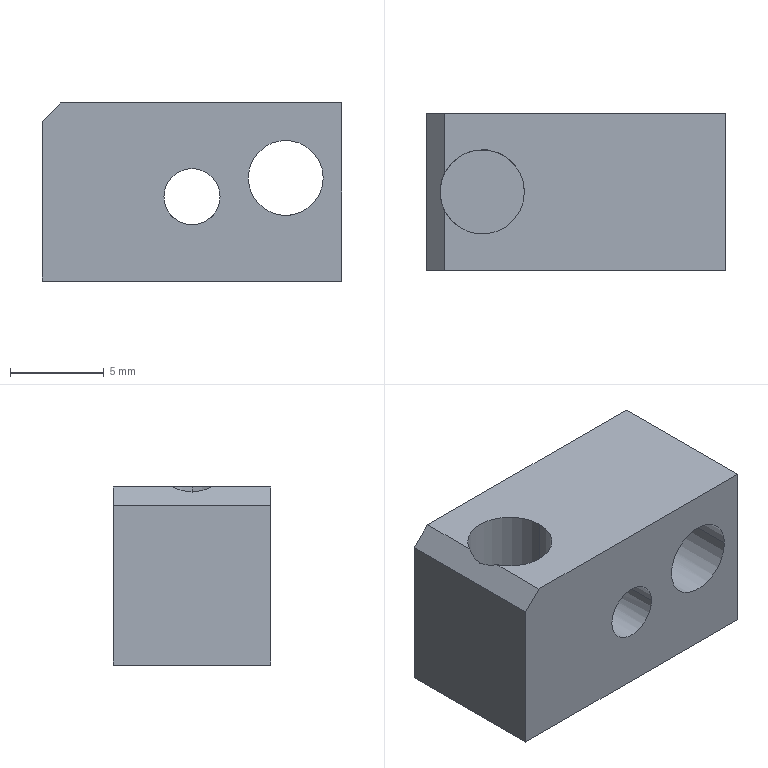Part | NX | 1 solid | 22 faces | box 16 x 8.4 x 9.5 mm | volume 978.124 mm3 | cylinder 10 | plane 8 | cone 4 | commonest cylinder face diameters 2.5 x4 3 x2 4 x2 4.5 x2
STEP:
#1=CARTESIAN_POINT('',(-8.,-4.2,-4.75));
#2=VERTEX_POINT('',#1);
#3=CARTESIAN_POINT('',(-8.,4.2,-4.75));
#4=VERTEX_POINT('',#3);
#5=CARTESIAN_POINT('',(-8.,0.,-4.75));
#6=DIRECTION('',(0.,1.,0.));
#7=VECTOR('',#6,1000.);
#8=LINE('',#5,#7);
#9=EDGE_CURVE('',#2,#4,#8,.T.);
#10=ORIENTED_EDGE('',*,*,#9,.T.);
#11=CARTESIAN_POINT('',(8.,4.2,-4.75));
#12=VERTEX_POINT('',#11);
#13=CARTESIAN_POINT('',(0.,4.2,-4.75));
#14=DIRECTION('',(1.,0.,0.));
#15=VECTOR('',#14,1000.);
#16=LINE('',#13,#15);
#17=EDGE_CURVE('',#4,#12,#16,.T.);
#18=ORIENTED_EDGE('',*,*,#17,.T.);
#19=CARTESIAN_POINT('',(8.,-4.2,-4.75));
#20=VERTEX_POINT('',#19);
#21=CARTESIAN_POINT('',(8.,0.,-4.75));
#22=DIRECTION('',(0.,-1.,0.));
#23=VECTOR('',#22,1000.);
#24=LINE('',#21,#23);
#25=EDGE_CURVE('',#12,#20,#24,.T.);
#26=ORIENTED_EDGE('',*,*,#25,.T.);
#27=CARTESIAN_POINT('',(0.,-4.2,-4.75));
#28=DIRECTION('',(-1.,0.,0.));
#29=VECTOR('',#28,1000.);
#30=LINE('',#27,#29);
#31=EDGE_CURVE('',#20,#2,#30,.T.);
#32=ORIENTED_EDGE('',*,*,#31,.T.);
#33=EDGE_LOOP('',(#10,#18,#26,#32));
#34=FACE_BOUND('',#33,.T.);
#35=CARTESIAN_POINT('',(3.3,0.,-4.75));
#36=VERTEX_POINT('',#35);
#37=CARTESIAN_POINT('',(6.7,0.,-4.75));
#38=VERTEX_POINT('',#37);
#39=CARTESIAN_POINT('',(5.,0.,-4.75));
#40=DIRECTION('',(0.,0.,-1.));
#41=DIRECTION('',(-1.,0.,0.));
#42=AXIS2_PLACEMENT_3D('',#39,#40,#41);
#43=CIRCLE('',#42,1.7);
#44=EDGE_CURVE('',#36,#38,#43,.T.);
#45=ORIENTED_EDGE('',*,*,#44,.F.);
#46=CARTESIAN_POINT('',(5.,0.,-4.75));
#47=DIRECTION('',(0.,0.,-1.));
#48=DIRECTION('',(-1.,0.,0.));
#49=AXIS2_PLACEMENT_3D('',#46,#47,#48);
#50=CIRCLE('',#49,1.7);
#51=EDGE_CURVE('',#38,#36,#50,.T.);
#52=ORIENTED_EDGE('',*,*,#51,.F.);
#53=EDGE_LOOP('',(#45,#52));
#54=FACE_BOUND('',#53,.T.);
#55=CARTESIAN_POINT('',(1.7,0.,-4.75));
#56=VERTEX_POINT('',#55);
#57=CARTESIAN_POINT('',(-1.7,0.,-4.75));
#58=VERTEX_POINT('',#57);
#59=CARTESIAN_POINT('',(0.,0.,-4.75));
#60=DIRECTION('',(0.,0.,-1.));
#61=DIRECTION('',(-1.,0.,0.));
#62=AXIS2_PLACEMENT_3D('',#59,#60,#61);
#63=CIRCLE('',#62,1.7);
#64=EDGE_CURVE('',#56,#58,#63,.T.);
#65=ORIENTED_EDGE('',*,*,#64,.F.);
#66=CARTESIAN_POINT('',(0.,0.,-4.75));
#67=DIRECTION('',(0.,0.,-1.));
#68=DIRECTION('',(-1.,0.,0.));
#69=AXIS2_PLACEMENT_3D('',#66,#67,#68);
#70=CIRCLE('',#69,1.7);
#71=EDGE_CURVE('',#58,#56,#70,.T.);
#72=ORIENTED_EDGE('',*,*,#71,.F.);
#73=EDGE_LOOP('',(#65,#72));
#74=FACE_BOUND('',#73,.T.);
#75=CARTESIAN_POINT('',(0.,0.,-4.75));
#76=DIRECTION('',(0.,0.,1.));
#77=DIRECTION('',(1.,0.,0.));
#78=AXIS2_PLACEMENT_3D('',#75,#76,#77);
#79=PLANE('',#78);
#80=ADVANCED_FACE('',(#34,#54,#74),#79,.F.);
#81=ORIENTED_EDGE('',*,*,#9,.F.);
#82=CARTESIAN_POINT('',(-8.,-4.2,3.75));
#83=VERTEX_POINT('',#82);
#84=CARTESIAN_POINT('',(-8.,-4.2,3.75));
#85=DIRECTION('',(0.,0.,-1.));
#86=VECTOR('',#85,1000.);
#87=LINE('',#84,#86);
#88=EDGE_CURVE('',#83,#2,#87,.T.);
#89=ORIENTED_EDGE('',*,*,#88,.F.);
#90=CARTESIAN_POINT('',(-8.,4.2,3.75));
#91=VERTEX_POINT('',#90);
#92=CARTESIAN_POINT('',(-8.,-4.2,3.75));
#93=DIRECTION('',(0.,1.,0.));
#94=VECTOR('',#93,1000.);
#95=LINE('',#92,#94);
#96=EDGE_CURVE('',#83,#91,#95,.T.);
#97=ORIENTED_EDGE('',*,*,#96,.T.);
#98=CARTESIAN_POINT('',(-8.,4.2,3.75));
#99=DIRECTION('',(0.,0.,-1.));
#100=VECTOR('',#99,1000.);
#101=LINE('',#98,#100);
#102=EDGE_CURVE('',#91,#4,#101,.T.);
#103=ORIENTED_EDGE('',*,*,#102,.T.);
#104=EDGE_LOOP('',(#81,#89,#97,#103));
#105=FACE_BOUND('',#104,.T.);
#106=CARTESIAN_POINT('',(-8.,4.2,-4.75));
#107=DIRECTION('',(-1.,0.,0.));
#108=DIRECTION('',(0.,0.,1.));
#109=AXIS2_PLACEMENT_3D('',#106,#107,#108);
#110=PLANE('',#109);
#111=ADVANCED_FACE('',(#105),#110,.T.);
#112=ORIENTED_EDGE('',*,*,#17,.F.);
#113=ORIENTED_EDGE('',*,*,#102,.F.);
#114=CARTESIAN_POINT('',(-7.,4.2,4.75));
#115=VERTEX_POINT('',#114);
#116=CARTESIAN_POINT('',(-7.,4.2,4.75));
#117=DIRECTION('',(-0.7071,0.,-0.7071));
#118=VECTOR('',#117,1000.);
#119=LINE('',#116,#118);
#120=EDGE_CURVE('',#115,#91,#119,.T.);
#121=ORIENTED_EDGE('',*,*,#120,.F.);
#122=CARTESIAN_POINT('',(8.,4.2,4.75));
#123=VERTEX_POINT('',#122);
#124=CARTESIAN_POINT('',(-7.,4.2,4.75));
#125=DIRECTION('',(1.,0.,0.));
#126=VECTOR('',#125,1000.);
#127=LINE('',#124,#126);
#128=EDGE_CURVE('',#115,#123,#127,.T.);
#129=ORIENTED_EDGE('',*,*,#128,.T.);
#130=CARTESIAN_POINT('',(8.,4.2,4.75));
#131=DIRECTION('',(0.,0.,-1.));
#132=VECTOR('',#131,1000.);
#133=LINE('',#130,#132);
#134=EDGE_CURVE('',#123,#12,#133,.T.);
#135=ORIENTED_EDGE('',*,*,#134,.T.);
#136=EDGE_LOOP('',(#112,#113,#121,#129,#135));
#137=FACE_BOUND('',#136,.T.);
#138=CARTESIAN_POINT('',(7.,4.2,0.75));
#139=VERTEX_POINT('',#138);
#140=CARTESIAN_POINT('',(3.,4.2,0.75));
#141=VERTEX_POINT('',#140);
#142=CARTESIAN_POINT('',(5.,4.2,0.75));
#143=DIRECTION('',(0.,1.,0.));
#144=DIRECTION('',(-1.,0.,0.));
#145=AXIS2_PLACEMENT_3D('',#142,#143,#144);
#146=CIRCLE('',#145,2.);
#147=EDGE_CURVE('',#139,#141,#146,.T.);
#148=ORIENTED_EDGE('',*,*,#147,.F.);
#149=CARTESIAN_POINT('',(5.,4.2,0.75));
#150=DIRECTION('',(0.,1.,0.));
#151=DIRECTION('',(-1.,0.,0.));
#152=AXIS2_PLACEMENT_3D('',#149,#150,#151);
#153=CIRCLE('',#152,2.);
#154=EDGE_CURVE('',#141,#139,#153,.T.);
#155=ORIENTED_EDGE('',*,*,#154,.F.);
#156=EDGE_LOOP('',(#148,#155));
#157=FACE_BOUND('',#156,.T.);
#158=CARTESIAN_POINT('',(-1.5,4.2,-0.25));
#159=VERTEX_POINT('',#158);
#160=CARTESIAN_POINT('',(1.5,4.2,-0.25));
#161=VERTEX_POINT('',#160);
#162=CARTESIAN_POINT('',(0.,4.2,-0.25));
#163=DIRECTION('',(0.,1.,0.));
#164=DIRECTION('',(-1.,0.,0.));
#165=AXIS2_PLACEMENT_3D('',#162,#163,#164);
#166=CIRCLE('',#165,1.5);
#167=EDGE_CURVE('',#159,#161,#166,.T.);
#168=ORIENTED_EDGE('',*,*,#167,.F.);
#169=CARTESIAN_POINT('',(0.,4.2,-0.25));
#170=DIRECTION('',(0.,1.,0.));
#171=DIRECTION('',(-1.,0.,0.));
#172=AXIS2_PLACEMENT_3D('',#169,#170,#171);
#173=CIRCLE('',#172,1.5);
#174=EDGE_CURVE('',#161,#159,#173,.T.);
#175=ORIENTED_EDGE('',*,*,#174,.F.);
#176=EDGE_LOOP('',(#168,#175));
#177=FACE_BOUND('',#176,.T.);
#178=CARTESIAN_POINT('',(8.,4.2,-4.75));
#179=DIRECTION('',(0.,1.,0.));
#180=DIRECTION('',(1.,0.,0.));
#181=AXIS2_PLACEMENT_3D('',#178,#179,#180);
#182=PLANE('',#181);
#183=ADVANCED_FACE('',(#137,#157,#177),#182,.T.);
#184=ORIENTED_EDGE('',*,*,#25,.F.);
#185=ORIENTED_EDGE('',*,*,#134,.F.);
#186=CARTESIAN_POINT('',(8.,-4.2,4.75));
#187=VERTEX_POINT('',#186);
#188=CARTESIAN_POINT('',(8.,4.2,4.75));
#189=DIRECTION('',(0.,-1.,0.));
#190=VECTOR('',#189,1000.);
#191=LINE('',#188,#190);
#192=EDGE_CURVE('',#123,#187,#191,.T.);
#193=ORIENTED_EDGE('',*,*,#192,.T.);
#194=CARTESIAN_POINT('',(8.,-4.2,4.75));
#195=DIRECTION('',(0.,0.,-1.));
#196=VECTOR('',#195,1000.);
#197=LINE('',#194,#196);
#198=EDGE_CURVE('',#187,#20,#197,.T.);
#199=ORIENTED_EDGE('',*,*,#198,.T.);
#200=EDGE_LOOP('',(#184,#185,#193,#199));
#201=FACE_BOUND('',#200,.T.);
#202=CARTESIAN_POINT('',(8.,-4.2,-4.75));
#203=DIRECTION('',(1.,0.,0.));
#204=DIRECTION('',(0.,1.,0.));
#205=AXIS2_PLACEMENT_3D('',#202,#203,#204);
#206=PLANE('',#205);
#207=ADVANCED_FACE('',(#201),#206,.T.);
#208=ORIENTED_EDGE('',*,*,#31,.F.);
#209=ORIENTED_EDGE('',*,*,#198,.F.);
#210=CARTESIAN_POINT('',(-7.,-4.2,4.75));
#211=VERTEX_POINT('',#210);
#212=CARTESIAN_POINT('',(8.,-4.2,4.75));
#213=DIRECTION('',(-1.,0.,0.));
#214=VECTOR('',#213,1000.);
#215=LINE('',#212,#214);
#216=EDGE_CURVE('',#187,#211,#215,.T.);
#217=ORIENTED_EDGE('',*,*,#216,.T.);
#218=CARTESIAN_POINT('',(-8.,-4.2,3.75));
#219=DIRECTION('',(0.7071,0.,0.7071));
#220=VECTOR('',#219,1000.);
#221=LINE('',#218,#220);
#222=EDGE_CURVE('',#83,#211,#221,.T.);
#223=ORIENTED_EDGE('',*,*,#222,.F.);
#224=ORIENTED_EDGE('',*,*,#88,.T.);
#225=EDGE_LOOP('',(#208,#209,#217,#223,#224));
#226=FACE_BOUND('',#225,.T.);
#227=CARTESIAN_POINT('',(7.,-4.2,0.75));
#228=VERTEX_POINT('',#227);
#229=CARTESIAN_POINT('',(3.,-4.2,0.75));
#230=VERTEX_POINT('',#229);
#231=CARTESIAN_POINT('',(5.,-4.2,0.75));
#232=DIRECTION('',(0.,1.,0.));
#233=DIRECTION('',(-1.,0.,0.));
#234=AXIS2_PLACEMENT_3D('',#231,#232,#233);
#235=CIRCLE('',#234,2.);
#236=EDGE_CURVE('',#228,#230,#235,.T.);
#237=ORIENTED_EDGE('',*,*,#236,.T.);
#238=CARTESIAN_POINT('',(5.,-4.2,0.75));
#239=DIRECTION('',(0.,1.,0.));
#240=DIRECTION('',(-1.,0.,0.));
#241=AXIS2_PLACEMENT_3D('',#238,#239,#240);
#242=CIRCLE('',#241,2.);
#243=EDGE_CURVE('',#230,#228,#242,.T.);
#244=ORIENTED_EDGE('',*,*,#243,.T.);
#245=EDGE_LOOP('',(#237,#244));
#246=FACE_BOUND('',#245,.T.);
#247=CARTESIAN_POINT('',(-1.5,-4.2,-0.25));
#248=VERTEX_POINT('',#247);
#249=CARTESIAN_POINT('',(1.5,-4.2,-0.25));
#250=VERTEX_POINT('',#249);
#251=CARTESIAN_POINT('',(0.,-4.2,-0.25));
#252=DIRECTION('',(0.,1.,0.));
#253=DIRECTION('',(-1.,0.,0.));
#254=AXIS2_PLACEMENT_3D('',#251,#252,#253);
#255=CIRCLE('',#254,1.5);
#256=EDGE_CURVE('',#248,#250,#255,.T.);
#257=ORIENTED_EDGE('',*,*,#256,.T.);
#258=CARTESIAN_POINT('',(0.,-4.2,-0.25));
#259=DIRECTION('',(0.,1.,0.));
#260=DIRECTION('',(-1.,0.,0.));
#261=AXIS2_PLACEMENT_3D('',#258,#259,#260);
#262=CIRCLE('',#261,1.5);
#263=EDGE_CURVE('',#250,#248,#262,.T.);
#264=ORIENTED_EDGE('',*,*,#263,.T.);
#265=EDGE_LOOP('',(#257,#264));
#266=FACE_BOUND('',#265,.T.);
#267=CARTESIAN_POINT('',(-8.,-4.2,-4.75));
#268=DIRECTION('',(0.,-1.,0.));
#269=DIRECTION('',(0.,0.,-1.));
#270=AXIS2_PLACEMENT_3D('',#267,#268,#269);
#271=PLANE('',#270);
#272=ADVANCED_FACE('',(#226,#246,#266),#271,.T.);
#273=CARTESIAN_POINT('',(-7.25,0.,4.5));
#274=VERTEX_POINT('',#273);
#275=CARTESIAN_POINT('',(-7.,-1.031,4.75));
#276=VERTEX_POINT('',#275);
#277=CARTESIAN_POINT('',(-7.,-1.031,4.75));
#278=CARTESIAN_POINT('',(-7.165,-0.7107,4.585));
#279=CARTESIAN_POINT('',(-7.25,-0.3538,4.5));
#280=CARTESIAN_POINT('',(-7.25,0.,4.5));
#281=B_SPLINE_CURVE_WITH_KNOTS('',3,(#277,#278,#279,#280),.UNSPECIFIED.,.F.,.F.,(4,4),(0.,1.),.UNSPECIFIED.);
#282=EDGE_CURVE('',#274,#276,#281,.F.);
#283=ORIENTED_EDGE('',*,*,#282,.F.);
#284=CARTESIAN_POINT('',(-7.,1.031,4.75));
#285=VERTEX_POINT('',#284);
#286=CARTESIAN_POINT('',(-7.25,0.,4.5));
#287=CARTESIAN_POINT('',(-7.25,0.3531,4.5));
#288=CARTESIAN_POINT('',(-7.165,0.7101,4.585));
#289=CARTESIAN_POINT('',(-7.,1.031,4.75));
#290=B_SPLINE_CURVE_WITH_KNOTS('',3,(#286,#287,#288,#289),.UNSPECIFIED.,.F.,.F.,(4,4),(0.,1.),.UNSPECIFIED.);
#291=EDGE_CURVE('',#285,#274,#290,.F.);
#292=ORIENTED_EDGE('',*,*,#291,.F.);
#293=CARTESIAN_POINT('',(-7.,1.031,4.75));
#294=DIRECTION('',(0.,1.,0.));
#295=VECTOR('',#294,1000.);
#296=LINE('',#293,#295);
#297=EDGE_CURVE('',#285,#115,#296,.T.);
#298=ORIENTED_EDGE('',*,*,#297,.T.);
#299=ORIENTED_EDGE('',*,*,#120,.T.);
#300=ORIENTED_EDGE('',*,*,#96,.F.);
#301=ORIENTED_EDGE('',*,*,#222,.T.);
#302=CARTESIAN_POINT('',(-7.,-4.2,4.75));
#303=DIRECTION('',(0.,1.,0.));
#304=VECTOR('',#303,1000.);
#305=LINE('',#302,#304);
#306=EDGE_CURVE('',#211,#276,#305,.T.);
#307=ORIENTED_EDGE('',*,*,#306,.T.);
#308=EDGE_LOOP('',(#283,#292,#298,#299,#300,#301,#307));
#309=FACE_BOUND('',#308,.T.);
#310=CARTESIAN_POINT('',(-7.,4.2,4.75));
#311=DIRECTION('',(0.7071,0.,-0.7071));
#312=DIRECTION('',(0.,-1.,0.));
#313=AXIS2_PLACEMENT_3D('',#310,#311,#312);
#314=PLANE('',#313);
#315=ADVANCED_FACE('',(#309),#314,.F.);
#316=ORIENTED_EDGE('',*,*,#291,.T.);
#317=CARTESIAN_POINT('',(-7.25,0.,-1.25));
#318=VERTEX_POINT('',#317);
#319=CARTESIAN_POINT('',(-7.25,0.,4.75));
#320=DIRECTION('',(0.,0.,-1.));
#321=VECTOR('',#320,1000.);
#322=LINE('',#319,#321);
#323=EDGE_CURVE('',#318,#274,#322,.F.);
#324=ORIENTED_EDGE('',*,*,#323,.F.);
#325=CARTESIAN_POINT('',(-2.75,0.,-1.25));
#326=VERTEX_POINT('',#325);
#327=CARTESIAN_POINT('',(-5.,0.,-1.25));
#328=DIRECTION('',(0.,0.,-1.));
#329=DIRECTION('',(-1.,0.,0.));
#330=AXIS2_PLACEMENT_3D('',#327,#328,#329);
#331=CIRCLE('',#330,2.25);
#332=EDGE_CURVE('',#318,#326,#331,.T.);
#333=ORIENTED_EDGE('',*,*,#332,.T.);
#334=CARTESIAN_POINT('',(-2.75,0.,4.75));
#335=VERTEX_POINT('',#334);
#336=CARTESIAN_POINT('',(-2.75,0.,4.75));
#337=DIRECTION('',(0.,0.,-1.));
#338=VECTOR('',#337,1000.);
#339=LINE('',#336,#338);
#340=EDGE_CURVE('',#326,#335,#339,.F.);
#341=ORIENTED_EDGE('',*,*,#340,.T.);
#342=CARTESIAN_POINT('',(-5.,0.,4.75));
#343=DIRECTION('',(0.,0.,1.));
#344=DIRECTION('',(-0.8889,-0.4581,0.));
#345=AXIS2_PLACEMENT_3D('',#342,#343,#344);
#346=CIRCLE('',#345,2.25);
#347=EDGE_CURVE('',#335,#285,#346,.T.);
#348=ORIENTED_EDGE('',*,*,#347,.T.);
#349=EDGE_LOOP('',(#316,#324,#333,#341,#348));
#350=FACE_BOUND('',#349,.T.);
#351=CARTESIAN_POINT('',(-5.,0.,4.75));
#352=DIRECTION('',(0.,0.,-1.));
#353=DIRECTION('',(-1.,0.,0.));
#354=AXIS2_PLACEMENT_3D('',#351,#352,#353);
#355=CYLINDRICAL_SURFACE('',#354,2.25);
#356=ADVANCED_FACE('',(#350),#355,.F.);
#357=ORIENTED_EDGE('',*,*,#167,.T.);
#358=CARTESIAN_POINT('',(1.5,-4.2,-0.25));
#359=DIRECTION('',(0.,1.,0.));
#360=VECTOR('',#359,1000.);
#361=LINE('',#358,#360);
#362=EDGE_CURVE('',#161,#250,#361,.F.);
#363=ORIENTED_EDGE('',*,*,#362,.T.);
#364=ORIENTED_EDGE('',*,*,#256,.F.);
#365=CARTESIAN_POINT('',(-1.5,-4.2,-0.25));
#366=DIRECTION('',(0.,1.,0.));
#367=VECTOR('',#366,1000.);
#368=LINE('',#365,#367);
#369=EDGE_CURVE('',#159,#248,#368,.F.);
#370=ORIENTED_EDGE('',*,*,#369,.F.);
#371=EDGE_LOOP('',(#357,#363,#364,#370));
#372=FACE_BOUND('',#371,.T.);
#373=CARTESIAN_POINT('',(0.,-4.2,-0.25));
#374=DIRECTION('',(0.,1.,0.));
#375=DIRECTION('',(-1.,0.,0.));
#376=AXIS2_PLACEMENT_3D('',#373,#374,#375);
#377=CYLINDRICAL_SURFACE('',#376,1.5);
#378=ADVANCED_FACE('',(#372),#377,.F.);
#379=ORIENTED_EDGE('',*,*,#347,.F.);
#380=CARTESIAN_POINT('',(-5.,0.,4.75));
#381=DIRECTION('',(0.,0.,1.));
#382=DIRECTION('',(-0.8889,-0.4581,0.));
#383=AXIS2_PLACEMENT_3D('',#380,#381,#382);
#384=CIRCLE('',#383,2.25);
#385=EDGE_CURVE('',#276,#335,#384,.T.);
#386=ORIENTED_EDGE('',*,*,#385,.F.);
#387=ORIENTED_EDGE('',*,*,#306,.F.);
#388=ORIENTED_EDGE('',*,*,#216,.F.);
#389=ORIENTED_EDGE('',*,*,#192,.F.);
#390=ORIENTED_EDGE('',*,*,#128,.F.);
#391=ORIENTED_EDGE('',*,*,#297,.F.);
#392=EDGE_LOOP('',(#379,#386,#387,#388,#389,#390,#391));
#393=FACE_BOUND('',#392,.T.);
#394=CARTESIAN_POINT('',(0.,0.,4.75));
#395=DIRECTION('',(0.,0.,1.));
#396=DIRECTION('',(1.,0.,0.));
#397=AXIS2_PLACEMENT_3D('',#394,#395,#396);
#398=PLANE('',#397);
#399=ADVANCED_FACE('',(#393),#398,.T.);
#400=CARTESIAN_POINT('',(-5.,0.,-1.25));
#401=DIRECTION('',(0.,0.,-1.));
#402=DIRECTION('',(-1.,0.,0.));
#403=AXIS2_PLACEMENT_3D('',#400,#401,#402);
#404=CIRCLE('',#403,2.25);
#405=EDGE_CURVE('',#326,#318,#404,.T.);
#406=ORIENTED_EDGE('',*,*,#405,.F.);
#407=ORIENTED_EDGE('',*,*,#332,.F.);
#408=EDGE_LOOP('',(#406,#407));
#409=FACE_BOUND('',#408,.T.);
#410=CARTESIAN_POINT('',(-5.,0.,-1.25));
#411=DIRECTION('',(0.,0.,-1.));
#412=DIRECTION('',(0.,-1.,0.));
#413=AXIS2_PLACEMENT_3D('',#410,#411,#412);
#414=PLANE('',#413);
#415=ADVANCED_FACE('',(#409),#414,.F.);
#416=ORIENTED_EDGE('',*,*,#236,.F.);
#417=CARTESIAN_POINT('',(7.,-4.2,0.75));
#418=DIRECTION('',(0.,1.,0.));
#419=VECTOR('',#418,1000.);
#420=LINE('',#417,#419);
#421=EDGE_CURVE('',#139,#228,#420,.F.);
#422=ORIENTED_EDGE('',*,*,#421,.F.);
#423=ORIENTED_EDGE('',*,*,#147,.T.);
#424=CARTESIAN_POINT('',(3.,-4.2,0.75));
#425=DIRECTION('',(0.,1.,0.));
#426=VECTOR('',#425,1000.);
#427=LINE('',#424,#426);
#428=EDGE_CURVE('',#141,#230,#427,.F.);
#429=ORIENTED_EDGE('',*,*,#428,.T.);
#430=EDGE_LOOP('',(#416,#422,#423,#429));
#431=FACE_BOUND('',#430,.T.);
#432=CARTESIAN_POINT('',(6.25,0.,-0.8112));
#433=VERTEX_POINT('',#432);
#434=CARTESIAN_POINT('',(3.75,0.,-0.8112));
#435=VERTEX_POINT('',#434);
#436=CARTESIAN_POINT('',(6.25,0.,-0.8112));
#437=CARTESIAN_POINT('',(6.25,-0.3293,-0.8115));
#438=CARTESIAN_POINT('',(5.984,-0.9739,-1.055));
#439=CARTESIAN_POINT('',(5.,-1.388,-1.347));
#440=CARTESIAN_POINT('',(4.017,-0.9746,-1.056));
#441=CARTESIAN_POINT('',(3.75,-0.3294,-0.8115));
#442=CARTESIAN_POINT('',(3.75,0.,-0.8112));
#443=B_SPLINE_CURVE_WITH_KNOTS('',3,(#436,#437,#438,#439,#440,#441,#442),.UNSPECIFIED.,.F.,.F.,(4,1,1,1,4),(0.,0.25,0.5,0.75,1.),.UNSPECIFIED.);
#444=EDGE_CURVE('',#433,#435,#443,.T.);
#445=ORIENTED_EDGE('',*,*,#444,.T.);
#446=CARTESIAN_POINT('',(3.75,0.,-0.8112));
#447=CARTESIAN_POINT('',(3.75,0.3294,-0.8115));
#448=CARTESIAN_POINT('',(4.017,0.9744,-1.056));
#449=CARTESIAN_POINT('',(5.,1.388,-1.347));
#450=CARTESIAN_POINT('',(5.983,0.974,-1.055));
#451=CARTESIAN_POINT('',(6.25,0.3294,-0.8115));
#452=CARTESIAN_POINT('',(6.25,0.,-0.8112));
#453=B_SPLINE_CURVE_WITH_KNOTS('',3,(#446,#447,#448,#449,#450,#451,#452),.UNSPECIFIED.,.F.,.F.,(4,1,1,1,4),(0.,0.25,0.5,0.75,1.),.UNSPECIFIED.);
#454=EDGE_CURVE('',#435,#433,#453,.T.);
#455=ORIENTED_EDGE('',*,*,#454,.T.);
#456=EDGE_LOOP('',(#445,#455));
#457=FACE_BOUND('',#456,.T.);
#458=CARTESIAN_POINT('',(5.,-4.2,0.75));
#459=DIRECTION('',(0.,1.,0.));
#460=DIRECTION('',(-1.,0.,0.));
#461=AXIS2_PLACEMENT_3D('',#458,#459,#460);
#462=CYLINDRICAL_SURFACE('',#461,2.);
#463=ADVANCED_FACE('',(#431,#457),#462,.F.);
#464=ORIENTED_EDGE('',*,*,#444,.F.);
#465=CARTESIAN_POINT('',(6.25,0.,-4.49));
#466=VERTEX_POINT('',#465);
#467=CARTESIAN_POINT('',(6.25,0.,-4.75));
#468=DIRECTION('',(0.,0.,-1.));
#469=VECTOR('',#468,1000.);
#470=LINE('',#467,#469);
#471=EDGE_CURVE('',#433,#466,#470,.T.);
#472=ORIENTED_EDGE('',*,*,#471,.T.);
#473=CARTESIAN_POINT('',(3.75,0.,-4.49));
#474=VERTEX_POINT('',#473);
#475=CARTESIAN_POINT('',(5.,0.,-4.49));
#476=DIRECTION('',(0.,0.,-1.));
#477=DIRECTION('',(-1.,0.,0.));
#478=AXIS2_PLACEMENT_3D('',#475,#476,#477);
#479=CIRCLE('',#478,1.25);
#480=EDGE_CURVE('',#466,#474,#479,.T.);
#481=ORIENTED_EDGE('',*,*,#480,.T.);
#482=CARTESIAN_POINT('',(3.75,0.,-4.75));
#483=DIRECTION('',(0.,0.,-1.));
#484=VECTOR('',#483,1000.);
#485=LINE('',#482,#484);
#486=EDGE_CURVE('',#435,#474,#485,.T.);
#487=ORIENTED_EDGE('',*,*,#486,.F.);
#488=EDGE_LOOP('',(#464,#472,#481,#487));
#489=FACE_BOUND('',#488,.T.);
#490=CARTESIAN_POINT('',(5.,0.,-4.75));
#491=DIRECTION('',(0.,0.,-1.));
#492=DIRECTION('',(-1.,0.,0.));
#493=AXIS2_PLACEMENT_3D('',#490,#491,#492);
#494=CYLINDRICAL_SURFACE('',#493,1.25);
#495=ADVANCED_FACE('',(#489),#494,.F.);
#496=CARTESIAN_POINT('',(5.,0.,-4.49));
#497=DIRECTION('',(0.,0.,-1.));
#498=DIRECTION('',(-1.,0.,0.));
#499=AXIS2_PLACEMENT_3D('',#496,#497,#498);
#500=CIRCLE('',#499,1.25);
#501=EDGE_CURVE('',#474,#466,#500,.T.);
#502=ORIENTED_EDGE('',*,*,#501,.F.);
#503=CARTESIAN_POINT('',(3.75,0.,-4.49));
#504=DIRECTION('',(-0.866,0.,-0.5));
#505=VECTOR('',#504,1000.);
#506=LINE('',#503,#505);
#507=EDGE_CURVE('',#36,#474,#506,.F.);
#508=ORIENTED_EDGE('',*,*,#507,.F.);
#509=ORIENTED_EDGE('',*,*,#44,.T.);
#510=CARTESIAN_POINT('',(6.25,0.,-4.49));
#511=DIRECTION('',(0.866,0.,-0.5));
#512=VECTOR('',#511,1000.);
#513=LINE('',#510,#512);
#514=EDGE_CURVE('',#38,#466,#513,.F.);
#515=ORIENTED_EDGE('',*,*,#514,.T.);
#516=EDGE_LOOP('',(#502,#508,#509,#515));
#517=FACE_BOUND('',#516,.T.);
#518=CARTESIAN_POINT('',(5.,0.,-4.49));
#519=DIRECTION('',(0.,0.,-1.));
#520=DIRECTION('',(-1.,0.,0.));
#521=AXIS2_PLACEMENT_3D('',#518,#519,#520);
#522=CONICAL_SURFACE('',#521,1.25,1.047);
#523=ADVANCED_FACE('',(#517),#522,.F.);
#524=CARTESIAN_POINT('',(-1.25,0.,-4.49));
#525=VERTEX_POINT('',#524);
#526=CARTESIAN_POINT('',(1.25,0.,-4.49));
#527=VERTEX_POINT('',#526);
#528=CARTESIAN_POINT('',(0.,0.,-4.49));
#529=DIRECTION('',(0.,0.,-1.));
#530=DIRECTION('',(-1.,0.,0.));
#531=AXIS2_PLACEMENT_3D('',#528,#529,#530);
#532=CIRCLE('',#531,1.25);
#533=EDGE_CURVE('',#525,#527,#532,.T.);
#534=ORIENTED_EDGE('',*,*,#533,.T.);
#535=CARTESIAN_POINT('',(1.25,0.,-1.079));
#536=VERTEX_POINT('',#535);
#537=CARTESIAN_POINT('',(1.25,0.,-4.75));
#538=DIRECTION('',(0.,0.,-1.));
#539=VECTOR('',#538,1000.);
#540=LINE('',#537,#539);
#541=EDGE_CURVE('',#527,#536,#540,.F.);
#542=ORIENTED_EDGE('',*,*,#541,.T.);
#543=CARTESIAN_POINT('',(-1.25,0.,-1.079));
#544=VERTEX_POINT('',#543);
#545=CARTESIAN_POINT('',(1.25,0.,-1.079));
#546=CARTESIAN_POINT('',(1.25,0.07277,-1.079));
#547=CARTESIAN_POINT('',(1.244,0.2201,-1.095));
#548=CARTESIAN_POINT('',(1.139,0.5219,-1.224));
#549=CARTESIAN_POINT('',(1.105,0.6124,-1.275));
#550=CARTESIAN_POINT('',(0.9097,0.8624,-1.444));
#551=CARTESIAN_POINT('',(0.9151,0.8524,-1.439));
#552=CARTESIAN_POINT('',(0.7904,0.9733,-1.527));
#553=CARTESIAN_POINT('',(0.6634,1.063,-1.597));
#554=CARTESIAN_POINT('',(0.4482,1.185,-1.696));
#555=CARTESIAN_POINT('',(-0.00003459,1.293,-1.786));
#556=CARTESIAN_POINT('',(-0.4481,1.185,-1.696));
#557=CARTESIAN_POINT('',(-0.6635,1.063,-1.597));
#558=CARTESIAN_POINT('',(-0.7907,0.9732,-1.527));
#559=CARTESIAN_POINT('',(-0.9153,0.8521,-1.439));
#560=CARTESIAN_POINT('',(-0.9103,0.8619,-1.444));
#561=CARTESIAN_POINT('',(-1.106,0.6121,-1.275));
#562=CARTESIAN_POINT('',(-1.14,0.5218,-1.224));
#563=CARTESIAN_POINT('',(-1.244,0.22,-1.095));
#564=CARTESIAN_POINT('',(-1.25,0.07274,-1.079));
#565=CARTESIAN_POINT('',(-1.25,0.,-1.079));
#566=B_SPLINE_CURVE_WITH_KNOTS('',3,(#545,#546,#547,#548,#549,#550,#551,#552,#553,#554,#555,#556,#557,#558,#559,#560,#561,#562,#563,#564,#565),.UNSPECIFIED.,.F.,.F.,(4,1,1,1,1,1,1,1,1,1,1,1,1,1,1,1,1,1,4),(0.,0.0625,0.125,0.1875,0.2188,0.25,0.2812,0.3125,0.375,0.5,0.625,0.6875,0.7188,0.75,0.7812,0.8125,0.875,0.9375,1.),.UNSPECIFIED.);
#567=EDGE_CURVE('',#544,#536,#566,.F.);
#568=ORIENTED_EDGE('',*,*,#567,.F.);
#569=CARTESIAN_POINT('',(-1.25,0.,-4.75));
#570=DIRECTION('',(0.,0.,-1.));
#571=VECTOR('',#570,1000.);
#572=LINE('',#569,#571);
#573=EDGE_CURVE('',#525,#544,#572,.F.);
#574=ORIENTED_EDGE('',*,*,#573,.F.);
#575=EDGE_LOOP('',(#534,#542,#568,#574));
#576=FACE_BOUND('',#575,.T.);
#577=CARTESIAN_POINT('',(0.,0.,-4.75));
#578=DIRECTION('',(0.,0.,-1.));
#579=DIRECTION('',(-1.,0.,0.));
#580=AXIS2_PLACEMENT_3D('',#577,#578,#579);
#581=CYLINDRICAL_SURFACE('',#580,1.25);
#582=ADVANCED_FACE('',(#576),#581,.F.);
#583=ORIENTED_EDGE('',*,*,#64,.T.);
#584=CARTESIAN_POINT('',(-1.25,0.,-4.49));
#585=DIRECTION('',(-0.866,0.,-0.5));
#586=VECTOR('',#585,1000.);
#587=LINE('',#584,#586);
#588=EDGE_CURVE('',#58,#525,#587,.F.);
#589=ORIENTED_EDGE('',*,*,#588,.T.);
#590=CARTESIAN_POINT('',(0.,0.,-4.49));
#591=DIRECTION('',(0.,0.,-1.));
#592=DIRECTION('',(-1.,0.,0.));
#593=AXIS2_PLACEMENT_3D('',#590,#591,#592);
#594=CIRCLE('',#593,1.25);
#595=EDGE_CURVE('',#527,#525,#594,.T.);
#596=ORIENTED_EDGE('',*,*,#595,.F.);
#597=CARTESIAN_POINT('',(1.25,0.,-4.49));
#598=DIRECTION('',(0.866,0.,-0.5));
#599=VECTOR('',#598,1000.);
#600=LINE('',#597,#599);
#601=EDGE_CURVE('',#56,#527,#600,.F.);
#602=ORIENTED_EDGE('',*,*,#601,.F.);
#603=EDGE_LOOP('',(#583,#589,#596,#602));
#604=FACE_BOUND('',#603,.T.);
#605=CARTESIAN_POINT('',(0.,0.,-4.49));
#606=DIRECTION('',(0.,0.,-1.));
#607=DIRECTION('',(-1.,0.,0.));
#608=AXIS2_PLACEMENT_3D('',#605,#606,#607);
#609=CONICAL_SURFACE('',#608,1.25,1.047);
#610=ADVANCED_FACE('',(#604),#609,.F.);
#611=ORIENTED_EDGE('',*,*,#507,.T.);
#612=ORIENTED_EDGE('',*,*,#480,.F.);
#613=ORIENTED_EDGE('',*,*,#514,.F.);
#614=ORIENTED_EDGE('',*,*,#51,.T.);
#615=EDGE_LOOP('',(#611,#612,#613,#614));
#616=FACE_BOUND('',#615,.T.);
#617=CARTESIAN_POINT('',(5.,0.,-4.49));
#618=DIRECTION('',(0.,0.,-1.));
#619=DIRECTION('',(-1.,0.,0.));
#620=AXIS2_PLACEMENT_3D('',#617,#618,#619);
#621=CONICAL_SURFACE('',#620,1.25,1.047);
#622=ADVANCED_FACE('',(#616),#621,.F.);
#623=ORIENTED_EDGE('',*,*,#405,.T.);
#624=ORIENTED_EDGE('',*,*,#323,.T.);
#625=ORIENTED_EDGE('',*,*,#282,.T.);
#626=ORIENTED_EDGE('',*,*,#385,.T.);
#627=ORIENTED_EDGE('',*,*,#340,.F.);
#628=EDGE_LOOP('',(#623,#624,#625,#626,#627));
#629=FACE_BOUND('',#628,.T.);
#630=CARTESIAN_POINT('',(-5.,0.,4.75));
#631=DIRECTION('',(0.,0.,-1.));
#632=DIRECTION('',(-1.,0.,0.));
#633=AXIS2_PLACEMENT_3D('',#630,#631,#632);
#634=CYLINDRICAL_SURFACE('',#633,2.25);
#635=ADVANCED_FACE('',(#629),#634,.F.);
#636=ORIENTED_EDGE('',*,*,#501,.T.);
#637=ORIENTED_EDGE('',*,*,#471,.F.);
#638=ORIENTED_EDGE('',*,*,#454,.F.);
#639=ORIENTED_EDGE('',*,*,#486,.T.);
#640=EDGE_LOOP('',(#636,#637,#638,#639));
#641=FACE_BOUND('',#640,.T.);
#642=CARTESIAN_POINT('',(5.,0.,-4.75));
#643=DIRECTION('',(0.,0.,-1.));
#644=DIRECTION('',(-1.,0.,0.));
#645=AXIS2_PLACEMENT_3D('',#642,#643,#644);
#646=CYLINDRICAL_SURFACE('',#645,1.25);
#647=ADVANCED_FACE('',(#641),#646,.F.);
#648=ORIENTED_EDGE('',*,*,#428,.F.);
#649=ORIENTED_EDGE('',*,*,#154,.T.);
#650=ORIENTED_EDGE('',*,*,#421,.T.);
#651=ORIENTED_EDGE('',*,*,#243,.F.);
#652=EDGE_LOOP('',(#648,#649,#650,#651));
#653=FACE_BOUND('',#652,.T.);
#654=CARTESIAN_POINT('',(5.,-4.2,0.75));
#655=DIRECTION('',(0.,1.,0.));
#656=DIRECTION('',(-1.,0.,0.));
#657=AXIS2_PLACEMENT_3D('',#654,#655,#656);
#658=CYLINDRICAL_SURFACE('',#657,2.);
#659=ADVANCED_FACE('',(#653),#658,.F.);
#660=ORIENTED_EDGE('',*,*,#533,.F.);
#661=ORIENTED_EDGE('',*,*,#588,.F.);
#662=ORIENTED_EDGE('',*,*,#71,.T.);
#663=ORIENTED_EDGE('',*,*,#601,.T.);
#664=EDGE_LOOP('',(#660,#661,#662,#663));
#665=FACE_BOUND('',#664,.T.);
#666=CARTESIAN_POINT('',(0.,0.,-4.49));
#667=DIRECTION('',(0.,0.,-1.));
#668=DIRECTION('',(-1.,0.,0.));
#669=AXIS2_PLACEMENT_3D('',#666,#667,#668);
#670=CONICAL_SURFACE('',#669,1.25,1.047);
#671=ADVANCED_FACE('',(#665),#670,.F.);
#672=ORIENTED_EDGE('',*,*,#573,.T.);
#673=CARTESIAN_POINT('',(-1.25,0.,-1.079));
#674=CARTESIAN_POINT('',(-1.25,-0.07273,-1.079));
#675=CARTESIAN_POINT('',(-1.244,-0.22,-1.095));
#676=CARTESIAN_POINT('',(-1.14,-0.5217,-1.224));
#677=CARTESIAN_POINT('',(-1.106,-0.6121,-1.275));
#678=CARTESIAN_POINT('',(-0.9099,-0.8623,-1.444));
#679=CARTESIAN_POINT('',(-0.9152,-0.8523,-1.439));
#680=CARTESIAN_POINT('',(-0.7906,-0.9732,-1.527));
#681=CARTESIAN_POINT('',(-0.6635,-1.062,-1.597));
#682=CARTESIAN_POINT('',(-0.4482,-1.185,-1.696));
#683=CARTESIAN_POINT('',(0.00003462,-1.293,-1.786));
#684=CARTESIAN_POINT('',(0.4481,-1.185,-1.696));
#685=CARTESIAN_POINT('',(0.6632,-1.063,-1.597));
#686=CARTESIAN_POINT('',(0.7904,-0.9734,-1.527));
#687=CARTESIAN_POINT('',(0.9151,-0.8525,-1.439));
#688=CARTESIAN_POINT('',(0.9101,-0.8621,-1.444));
#689=CARTESIAN_POINT('',(1.105,-0.6126,-1.275));
#690=CARTESIAN_POINT('',(1.139,-0.522,-1.224));
#691=CARTESIAN_POINT('',(1.244,-0.2202,-1.095));
#692=CARTESIAN_POINT('',(1.25,-0.07279,-1.079));
#693=CARTESIAN_POINT('',(1.25,0.,-1.079));
#694=B_SPLINE_CURVE_WITH_KNOTS('',3,(#673,#674,#675,#676,#677,#678,#679,#680,#681,#682,#683,#684,#685,#686,#687,#688,#689,#690,#691,#692,#693),.UNSPECIFIED.,.F.,.F.,(4,1,1,1,1,1,1,1,1,1,1,1,1,1,1,1,1,1,4),(0.,0.0625,0.125,0.1875,0.2188,0.25,0.2812,0.3125,0.375,0.5,0.625,0.6875,0.7188,0.75,0.7812,0.8125,0.875,0.9375,1.),.UNSPECIFIED.);
#695=EDGE_CURVE('',#536,#544,#694,.F.);
#696=ORIENTED_EDGE('',*,*,#695,.F.);
#697=ORIENTED_EDGE('',*,*,#541,.F.);
#698=ORIENTED_EDGE('',*,*,#595,.T.);
#699=EDGE_LOOP('',(#672,#696,#697,#698));
#700=FACE_BOUND('',#699,.T.);
#701=CARTESIAN_POINT('',(0.,0.,-4.75));
#702=DIRECTION('',(0.,0.,-1.));
#703=DIRECTION('',(-1.,0.,0.));
#704=AXIS2_PLACEMENT_3D('',#701,#702,#703);
#705=CYLINDRICAL_SURFACE('',#704,1.25);
#706=ADVANCED_FACE('',(#700),#705,.F.);
#707=ORIENTED_EDGE('',*,*,#369,.T.);
#708=ORIENTED_EDGE('',*,*,#263,.F.);
#709=ORIENTED_EDGE('',*,*,#362,.F.);
#710=ORIENTED_EDGE('',*,*,#174,.T.);
#711=EDGE_LOOP('',(#707,#708,#709,#710));
#712=FACE_BOUND('',#711,.T.);
#713=ORIENTED_EDGE('',*,*,#567,.T.);
#714=ORIENTED_EDGE('',*,*,#695,.T.);
#715=EDGE_LOOP('',(#713,#714));
#716=FACE_BOUND('',#715,.T.);
#717=CARTESIAN_POINT('',(0.,-4.2,-0.25));
#718=DIRECTION('',(0.,1.,0.));
#719=DIRECTION('',(-1.,0.,0.));
#720=AXIS2_PLACEMENT_3D('',#717,#718,#719);
#721=CYLINDRICAL_SURFACE('',#720,1.5);
#722=ADVANCED_FACE('',(#712,#716),#721,.F.);
#723=CLOSED_SHELL('',(#80,#111,#183,#207,#272,#315,#356,#378,#399,#415,#463,#495,#523,#582,#610,#622,#635,#647,#659,#671,#706,#722));
#724=MANIFOLD_SOLID_BREP('',#723);
#725=(LENGTH_UNIT()NAMED_UNIT(*)SI_UNIT(.MILLI.,.METRE.));
#726=UNCERTAINTY_MEASURE_WITH_UNIT(LENGTH_MEASURE(0.0508),#725,'','');
#727=(NAMED_UNIT(*)PLANE_ANGLE_UNIT()SI_UNIT($,.RADIAN.));
#728=(NAMED_UNIT(*)SI_UNIT($,.STERADIAN.)SOLID_ANGLE_UNIT());
#729=(GEOMETRIC_REPRESENTATION_CONTEXT(3)GLOBAL_UNCERTAINTY_ASSIGNED_CONTEXT((#726))GLOBAL_UNIT_ASSIGNED_CONTEXT((#725,#727,#728))REPRESENTATION_CONTEXT('',''));
#730=ADVANCED_BREP_SHAPE_REPRESENTATION('',(#724),#729);